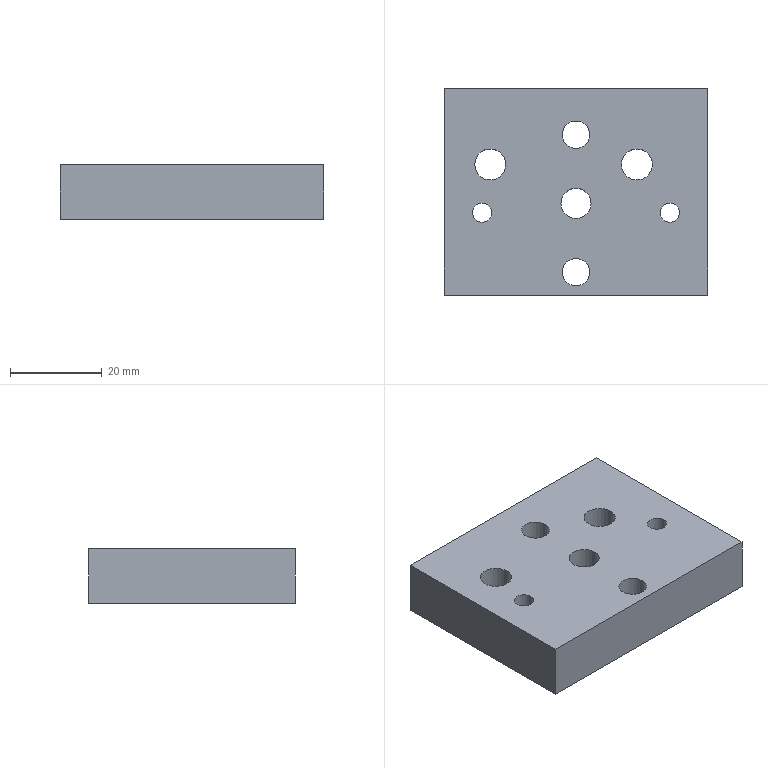Part | NX | features BREP 1 | 1 solid | 15 faces | box 57.5 x 45 x 12 mm | volume 28368 mm3 | cylinder 8 | plane 7 | commonest cylinder face diameters 4.2 x2 6 x2 6.8 x2 6.6 x1 11 x1
STEP:
#1=CARTESIAN_POINT('',(28.75,-22.5,0.));
#2=VERTEX_POINT('',#1);
#3=CARTESIAN_POINT('',(28.75,22.5,0.));
#4=VERTEX_POINT('',#3);
#5=CARTESIAN_POINT('',(28.75,22.5,0.));
#6=DIRECTION('',(0.,1.,0.));
#7=VECTOR('',#6,1000.);
#8=LINE('',#5,#7);
#9=EDGE_CURVE('',#2,#4,#8,.T.);
#10=ORIENTED_EDGE('',*,*,#9,.T.);
#11=CARTESIAN_POINT('',(28.75,22.5,12.));
#12=VERTEX_POINT('',#11);
#13=CARTESIAN_POINT('',(28.75,22.5,12.));
#14=DIRECTION('',(0.,0.,-1.));
#15=VECTOR('',#14,1000.);
#16=LINE('',#13,#15);
#17=EDGE_CURVE('',#12,#4,#16,.T.);
#18=ORIENTED_EDGE('',*,*,#17,.F.);
#19=CARTESIAN_POINT('',(28.75,-22.5,12.));
#20=VERTEX_POINT('',#19);
#21=CARTESIAN_POINT('',(28.75,22.5,12.));
#22=DIRECTION('',(0.,1.,0.));
#23=VECTOR('',#22,1000.);
#24=LINE('',#21,#23);
#25=EDGE_CURVE('',#20,#12,#24,.T.);
#26=ORIENTED_EDGE('',*,*,#25,.F.);
#27=CARTESIAN_POINT('',(28.75,-22.5,12.));
#28=DIRECTION('',(0.,0.,-1.));
#29=VECTOR('',#28,1000.);
#30=LINE('',#27,#29);
#31=EDGE_CURVE('',#20,#2,#30,.T.);
#32=ORIENTED_EDGE('',*,*,#31,.T.);
#33=EDGE_LOOP('',(#10,#18,#26,#32));
#34=FACE_BOUND('',#33,.T.);
#35=CARTESIAN_POINT('',(28.75,22.5,12.));
#36=DIRECTION('',(-1.,0.,0.));
#37=DIRECTION('',(0.,1.,0.));
#38=AXIS2_PLACEMENT_3D('',#35,#36,#37);
#39=PLANE('',#38);
#40=ADVANCED_FACE('',(#34),#39,.F.);
#41=CARTESIAN_POINT('',(-28.75,22.5,0.));
#42=VERTEX_POINT('',#41);
#43=CARTESIAN_POINT('',(-28.75,22.5,0.));
#44=DIRECTION('',(-1.,0.,0.));
#45=VECTOR('',#44,1000.);
#46=LINE('',#43,#45);
#47=EDGE_CURVE('',#4,#42,#46,.T.);
#48=ORIENTED_EDGE('',*,*,#47,.T.);
#49=CARTESIAN_POINT('',(-28.75,22.5,12.));
#50=VERTEX_POINT('',#49);
#51=CARTESIAN_POINT('',(-28.75,22.5,12.));
#52=DIRECTION('',(0.,0.,-1.));
#53=VECTOR('',#52,1000.);
#54=LINE('',#51,#53);
#55=EDGE_CURVE('',#50,#42,#54,.T.);
#56=ORIENTED_EDGE('',*,*,#55,.F.);
#57=CARTESIAN_POINT('',(-28.75,22.5,12.));
#58=DIRECTION('',(-1.,0.,0.));
#59=VECTOR('',#58,1000.);
#60=LINE('',#57,#59);
#61=EDGE_CURVE('',#12,#50,#60,.T.);
#62=ORIENTED_EDGE('',*,*,#61,.F.);
#63=ORIENTED_EDGE('',*,*,#17,.T.);
#64=EDGE_LOOP('',(#48,#56,#62,#63));
#65=FACE_BOUND('',#64,.T.);
#66=CARTESIAN_POINT('',(-28.75,22.5,12.));
#67=DIRECTION('',(0.,-1.,0.));
#68=DIRECTION('',(0.,0.,1.));
#69=AXIS2_PLACEMENT_3D('',#66,#67,#68);
#70=PLANE('',#69);
#71=ADVANCED_FACE('',(#65),#70,.F.);
#72=CARTESIAN_POINT('',(-28.75,-22.5,0.));
#73=VERTEX_POINT('',#72);
#74=CARTESIAN_POINT('',(-28.75,22.5,0.));
#75=DIRECTION('',(0.,-1.,0.));
#76=VECTOR('',#75,1000.);
#77=LINE('',#74,#76);
#78=EDGE_CURVE('',#42,#73,#77,.T.);
#79=ORIENTED_EDGE('',*,*,#78,.T.);
#80=CARTESIAN_POINT('',(-28.75,-22.5,12.));
#81=VERTEX_POINT('',#80);
#82=CARTESIAN_POINT('',(-28.75,-22.5,12.));
#83=DIRECTION('',(0.,0.,-1.));
#84=VECTOR('',#83,1000.);
#85=LINE('',#82,#84);
#86=EDGE_CURVE('',#81,#73,#85,.T.);
#87=ORIENTED_EDGE('',*,*,#86,.F.);
#88=CARTESIAN_POINT('',(-28.75,22.5,12.));
#89=DIRECTION('',(0.,-1.,0.));
#90=VECTOR('',#89,1000.);
#91=LINE('',#88,#90);
#92=EDGE_CURVE('',#50,#81,#91,.T.);
#93=ORIENTED_EDGE('',*,*,#92,.F.);
#94=ORIENTED_EDGE('',*,*,#55,.T.);
#95=EDGE_LOOP('',(#79,#87,#93,#94));
#96=FACE_BOUND('',#95,.T.);
#97=CARTESIAN_POINT('',(-28.75,22.5,12.));
#98=DIRECTION('',(1.,0.,0.));
#99=DIRECTION('',(0.,-1.,0.));
#100=AXIS2_PLACEMENT_3D('',#97,#98,#99);
#101=PLANE('',#100);
#102=ADVANCED_FACE('',(#96),#101,.F.);
#103=CARTESIAN_POINT('',(-28.75,-22.5,0.));
#104=DIRECTION('',(1.,0.,0.));
#105=VECTOR('',#104,1000.);
#106=LINE('',#103,#105);
#107=EDGE_CURVE('',#73,#2,#106,.T.);
#108=ORIENTED_EDGE('',*,*,#107,.T.);
#109=ORIENTED_EDGE('',*,*,#31,.F.);
#110=CARTESIAN_POINT('',(-28.75,-22.5,12.));
#111=DIRECTION('',(1.,0.,0.));
#112=VECTOR('',#111,1000.);
#113=LINE('',#110,#112);
#114=EDGE_CURVE('',#81,#20,#113,.T.);
#115=ORIENTED_EDGE('',*,*,#114,.F.);
#116=ORIENTED_EDGE('',*,*,#86,.T.);
#117=EDGE_LOOP('',(#108,#109,#115,#116));
#118=FACE_BOUND('',#117,.T.);
#119=CARTESIAN_POINT('',(-28.75,-22.5,12.));
#120=DIRECTION('',(0.,1.,0.));
#121=DIRECTION('',(0.,0.,-1.));
#122=AXIS2_PLACEMENT_3D('',#119,#120,#121);
#123=PLANE('',#122);
#124=ADVANCED_FACE('',(#118),#123,.F.);
#125=CARTESIAN_POINT('',(-3.3,-2.5,12.));
#126=VERTEX_POINT('',#125);
#127=CARTESIAN_POINT('',(0.,-2.5,12.));
#128=DIRECTION('',(0.,0.,-1.));
#129=DIRECTION('',(-1.,0.,0.));
#130=AXIS2_PLACEMENT_3D('',#127,#128,#129);
#131=CIRCLE('',#130,3.3);
#132=EDGE_CURVE('',#126,#126,#131,.T.);
#133=ORIENTED_EDGE('',*,*,#132,.T.);
#134=EDGE_LOOP('',(#133));
#135=FACE_BOUND('',#134,.T.);
#136=CARTESIAN_POINT('',(-3.,-17.5,12.));
#137=VERTEX_POINT('',#136);
#138=CARTESIAN_POINT('',(0.,-17.5,12.));
#139=DIRECTION('',(0.,0.,-1.));
#140=DIRECTION('',(-1.,0.,0.));
#141=AXIS2_PLACEMENT_3D('',#138,#139,#140);
#142=CIRCLE('',#141,3.);
#143=EDGE_CURVE('',#137,#137,#142,.T.);
#144=ORIENTED_EDGE('',*,*,#143,.T.);
#145=EDGE_LOOP('',(#144));
#146=FACE_BOUND('',#145,.T.);
#147=CARTESIAN_POINT('',(-3.,12.5,12.));
#148=VERTEX_POINT('',#147);
#149=CARTESIAN_POINT('',(0.,12.5,12.));
#150=DIRECTION('',(0.,0.,-1.));
#151=DIRECTION('',(-1.,0.,0.));
#152=AXIS2_PLACEMENT_3D('',#149,#150,#151);
#153=CIRCLE('',#152,3.);
#154=EDGE_CURVE('',#148,#148,#153,.T.);
#155=ORIENTED_EDGE('',*,*,#154,.T.);
#156=EDGE_LOOP('',(#155));
#157=FACE_BOUND('',#156,.T.);
#158=CARTESIAN_POINT('',(-18.4,-4.5,12.));
#159=VERTEX_POINT('',#158);
#160=CARTESIAN_POINT('',(-20.5,-4.5,12.));
#161=DIRECTION('',(0.,0.,1.));
#162=DIRECTION('',(1.,0.,0.));
#163=AXIS2_PLACEMENT_3D('',#160,#161,#162);
#164=CIRCLE('',#163,2.1);
#165=EDGE_CURVE('',#159,#159,#164,.T.);
#166=ORIENTED_EDGE('',*,*,#165,.F.);
#167=EDGE_LOOP('',(#166));
#168=FACE_BOUND('',#167,.T.);
#169=CARTESIAN_POINT('',(22.6,-4.5,12.));
#170=VERTEX_POINT('',#169);
#171=CARTESIAN_POINT('',(20.5,-4.5,12.));
#172=DIRECTION('',(0.,0.,1.));
#173=DIRECTION('',(1.,0.,0.));
#174=AXIS2_PLACEMENT_3D('',#171,#172,#173);
#175=CIRCLE('',#174,2.1);
#176=EDGE_CURVE('',#170,#170,#175,.T.);
#177=ORIENTED_EDGE('',*,*,#176,.F.);
#178=EDGE_LOOP('',(#177));
#179=FACE_BOUND('',#178,.T.);
#180=CARTESIAN_POINT('',(9.886,6.,12.));
#181=VERTEX_POINT('',#180);
#182=CARTESIAN_POINT('',(13.286,6.,12.));
#183=DIRECTION('',(0.,0.,-1.));
#184=DIRECTION('',(-1.,0.,0.));
#185=AXIS2_PLACEMENT_3D('',#182,#183,#184);
#186=CIRCLE('',#185,3.4);
#187=EDGE_CURVE('',#181,#181,#186,.T.);
#188=ORIENTED_EDGE('',*,*,#187,.T.);
#189=EDGE_LOOP('',(#188));
#190=FACE_BOUND('',#189,.T.);
#191=CARTESIAN_POINT('',(-22.114,6.,12.));
#192=VERTEX_POINT('',#191);
#193=CARTESIAN_POINT('',(-18.714,6.,12.));
#194=DIRECTION('',(0.,0.,-1.));
#195=DIRECTION('',(-1.,0.,0.));
#196=AXIS2_PLACEMENT_3D('',#193,#194,#195);
#197=CIRCLE('',#196,3.4);
#198=EDGE_CURVE('',#192,#192,#197,.T.);
#199=ORIENTED_EDGE('',*,*,#198,.T.);
#200=EDGE_LOOP('',(#199));
#201=FACE_BOUND('',#200,.T.);
#202=ORIENTED_EDGE('',*,*,#25,.T.);
#203=ORIENTED_EDGE('',*,*,#61,.T.);
#204=ORIENTED_EDGE('',*,*,#92,.T.);
#205=ORIENTED_EDGE('',*,*,#114,.T.);
#206=EDGE_LOOP('',(#202,#203,#204,#205));
#207=FACE_BOUND('',#206,.T.);
#208=CARTESIAN_POINT('',(0.,0.,12.));
#209=DIRECTION('',(0.,0.,1.));
#210=DIRECTION('',(-1.,0.,0.));
#211=AXIS2_PLACEMENT_3D('',#208,#209,#210);
#212=PLANE('',#211);
#213=ADVANCED_FACE('',(#135,#146,#157,#168,#179,#190,#201,#207),#212,.T.);
#214=CARTESIAN_POINT('',(-5.5,-2.5,0.));
#215=VERTEX_POINT('',#214);
#216=CARTESIAN_POINT('',(0.,-2.5,0.));
#217=DIRECTION('',(0.,0.,-1.));
#218=DIRECTION('',(-1.,0.,0.));
#219=AXIS2_PLACEMENT_3D('',#216,#217,#218);
#220=CIRCLE('',#219,5.5);
#221=EDGE_CURVE('',#215,#215,#220,.T.);
#222=ORIENTED_EDGE('',*,*,#221,.F.);
#223=EDGE_LOOP('',(#222));
#224=FACE_BOUND('',#223,.T.);
#225=CARTESIAN_POINT('',(-3.,-17.5,0.));
#226=VERTEX_POINT('',#225);
#227=CARTESIAN_POINT('',(0.,-17.5,0.));
#228=DIRECTION('',(0.,0.,-1.));
#229=DIRECTION('',(-1.,0.,0.));
#230=AXIS2_PLACEMENT_3D('',#227,#228,#229);
#231=CIRCLE('',#230,3.);
#232=EDGE_CURVE('',#226,#226,#231,.T.);
#233=ORIENTED_EDGE('',*,*,#232,.F.);
#234=EDGE_LOOP('',(#233));
#235=FACE_BOUND('',#234,.T.);
#236=CARTESIAN_POINT('',(-3.,12.5,0.));
#237=VERTEX_POINT('',#236);
#238=CARTESIAN_POINT('',(0.,12.5,0.));
#239=DIRECTION('',(0.,0.,-1.));
#240=DIRECTION('',(-1.,0.,0.));
#241=AXIS2_PLACEMENT_3D('',#238,#239,#240);
#242=CIRCLE('',#241,3.);
#243=EDGE_CURVE('',#237,#237,#242,.T.);
#244=ORIENTED_EDGE('',*,*,#243,.F.);
#245=EDGE_LOOP('',(#244));
#246=FACE_BOUND('',#245,.T.);
#247=CARTESIAN_POINT('',(-18.4,-4.5,0.));
#248=VERTEX_POINT('',#247);
#249=CARTESIAN_POINT('',(-20.5,-4.5,0.));
#250=DIRECTION('',(0.,0.,1.));
#251=DIRECTION('',(1.,0.,0.));
#252=AXIS2_PLACEMENT_3D('',#249,#250,#251);
#253=CIRCLE('',#252,2.1);
#254=EDGE_CURVE('',#248,#248,#253,.T.);
#255=ORIENTED_EDGE('',*,*,#254,.T.);
#256=EDGE_LOOP('',(#255));
#257=FACE_BOUND('',#256,.T.);
#258=CARTESIAN_POINT('',(22.6,-4.5,0.));
#259=VERTEX_POINT('',#258);
#260=CARTESIAN_POINT('',(20.5,-4.5,0.));
#261=DIRECTION('',(0.,0.,1.));
#262=DIRECTION('',(1.,0.,0.));
#263=AXIS2_PLACEMENT_3D('',#260,#261,#262);
#264=CIRCLE('',#263,2.1);
#265=EDGE_CURVE('',#259,#259,#264,.T.);
#266=ORIENTED_EDGE('',*,*,#265,.T.);
#267=EDGE_LOOP('',(#266));
#268=FACE_BOUND('',#267,.T.);
#269=CARTESIAN_POINT('',(9.886,6.,0.));
#270=VERTEX_POINT('',#269);
#271=CARTESIAN_POINT('',(13.286,6.,0.));
#272=DIRECTION('',(0.,0.,-1.));
#273=DIRECTION('',(-1.,0.,0.));
#274=AXIS2_PLACEMENT_3D('',#271,#272,#273);
#275=CIRCLE('',#274,3.4);
#276=EDGE_CURVE('',#270,#270,#275,.T.);
#277=ORIENTED_EDGE('',*,*,#276,.F.);
#278=EDGE_LOOP('',(#277));
#279=FACE_BOUND('',#278,.T.);
#280=CARTESIAN_POINT('',(-22.114,6.,0.));
#281=VERTEX_POINT('',#280);
#282=CARTESIAN_POINT('',(-18.714,6.,0.));
#283=DIRECTION('',(0.,0.,-1.));
#284=DIRECTION('',(-1.,0.,0.));
#285=AXIS2_PLACEMENT_3D('',#282,#283,#284);
#286=CIRCLE('',#285,3.4);
#287=EDGE_CURVE('',#281,#281,#286,.T.);
#288=ORIENTED_EDGE('',*,*,#287,.F.);
#289=EDGE_LOOP('',(#288));
#290=FACE_BOUND('',#289,.T.);
#291=ORIENTED_EDGE('',*,*,#9,.F.);
#292=ORIENTED_EDGE('',*,*,#107,.F.);
#293=ORIENTED_EDGE('',*,*,#78,.F.);
#294=ORIENTED_EDGE('',*,*,#47,.F.);
#295=EDGE_LOOP('',(#291,#292,#293,#294));
#296=FACE_BOUND('',#295,.T.);
#297=CARTESIAN_POINT('',(0.,0.,0.));
#298=DIRECTION('',(0.,0.,1.));
#299=DIRECTION('',(-1.,0.,0.));
#300=AXIS2_PLACEMENT_3D('',#297,#298,#299);
#301=PLANE('',#300);
#302=ADVANCED_FACE('',(#224,#235,#246,#257,#268,#279,#290,#296),#301,.F.);
#303=ORIENTED_EDGE('',*,*,#198,.F.);
#304=EDGE_LOOP('',(#303));
#305=FACE_BOUND('',#304,.T.);
#306=ORIENTED_EDGE('',*,*,#287,.T.);
#307=EDGE_LOOP('',(#306));
#308=FACE_BOUND('',#307,.T.);
#309=CARTESIAN_POINT('',(-18.714,6.,0.));
#310=DIRECTION('',(0.,0.,-1.));
#311=DIRECTION('',(1.,0.,0.));
#312=AXIS2_PLACEMENT_3D('',#309,#310,#311);
#313=CYLINDRICAL_SURFACE('',#312,3.4);
#314=ADVANCED_FACE('',(#305,#308),#313,.F.);
#315=ORIENTED_EDGE('',*,*,#187,.F.);
#316=EDGE_LOOP('',(#315));
#317=FACE_BOUND('',#316,.T.);
#318=ORIENTED_EDGE('',*,*,#276,.T.);
#319=EDGE_LOOP('',(#318));
#320=FACE_BOUND('',#319,.T.);
#321=CARTESIAN_POINT('',(13.286,6.,0.));
#322=DIRECTION('',(0.,0.,-1.));
#323=DIRECTION('',(1.,0.,0.));
#324=AXIS2_PLACEMENT_3D('',#321,#322,#323);
#325=CYLINDRICAL_SURFACE('',#324,3.4);
#326=ADVANCED_FACE('',(#317,#320),#325,.F.);
#327=ORIENTED_EDGE('',*,*,#265,.F.);
#328=EDGE_LOOP('',(#327));
#329=FACE_BOUND('',#328,.T.);
#330=ORIENTED_EDGE('',*,*,#176,.T.);
#331=EDGE_LOOP('',(#330));
#332=FACE_BOUND('',#331,.T.);
#333=CARTESIAN_POINT('',(20.5,-4.5,12.));
#334=DIRECTION('',(0.,0.,1.));
#335=DIRECTION('',(-1.,0.,0.));
#336=AXIS2_PLACEMENT_3D('',#333,#334,#335);
#337=CYLINDRICAL_SURFACE('',#336,2.1);
#338=ADVANCED_FACE('',(#329,#332),#337,.F.);
#339=ORIENTED_EDGE('',*,*,#254,.F.);
#340=EDGE_LOOP('',(#339));
#341=FACE_BOUND('',#340,.T.);
#342=ORIENTED_EDGE('',*,*,#165,.T.);
#343=EDGE_LOOP('',(#342));
#344=FACE_BOUND('',#343,.T.);
#345=CARTESIAN_POINT('',(-20.5,-4.5,12.));
#346=DIRECTION('',(0.,0.,1.));
#347=DIRECTION('',(-1.,0.,0.));
#348=AXIS2_PLACEMENT_3D('',#345,#346,#347);
#349=CYLINDRICAL_SURFACE('',#348,2.1);
#350=ADVANCED_FACE('',(#341,#344),#349,.F.);
#351=ORIENTED_EDGE('',*,*,#154,.F.);
#352=EDGE_LOOP('',(#351));
#353=FACE_BOUND('',#352,.T.);
#354=ORIENTED_EDGE('',*,*,#243,.T.);
#355=EDGE_LOOP('',(#354));
#356=FACE_BOUND('',#355,.T.);
#357=CARTESIAN_POINT('',(0.,12.5,0.));
#358=DIRECTION('',(0.,0.,-1.));
#359=DIRECTION('',(1.,0.,0.));
#360=AXIS2_PLACEMENT_3D('',#357,#358,#359);
#361=CYLINDRICAL_SURFACE('',#360,3.);
#362=ADVANCED_FACE('',(#353,#356),#361,.F.);
#363=ORIENTED_EDGE('',*,*,#143,.F.);
#364=EDGE_LOOP('',(#363));
#365=FACE_BOUND('',#364,.T.);
#366=ORIENTED_EDGE('',*,*,#232,.T.);
#367=EDGE_LOOP('',(#366));
#368=FACE_BOUND('',#367,.T.);
#369=CARTESIAN_POINT('',(0.,-17.5,0.));
#370=DIRECTION('',(0.,0.,-1.));
#371=DIRECTION('',(1.,0.,0.));
#372=AXIS2_PLACEMENT_3D('',#369,#370,#371);
#373=CYLINDRICAL_SURFACE('',#372,3.);
#374=ADVANCED_FACE('',(#365,#368),#373,.F.);
#375=ORIENTED_EDGE('',*,*,#132,.F.);
#376=EDGE_LOOP('',(#375));
#377=FACE_BOUND('',#376,.T.);
#378=CARTESIAN_POINT('',(-3.3,-2.5,6.4));
#379=VERTEX_POINT('',#378);
#380=CARTESIAN_POINT('',(0.,-2.5,6.4));
#381=DIRECTION('',(0.,0.,-1.));
#382=DIRECTION('',(-1.,0.,0.));
#383=AXIS2_PLACEMENT_3D('',#380,#381,#382);
#384=CIRCLE('',#383,3.3);
#385=EDGE_CURVE('',#379,#379,#384,.T.);
#386=ORIENTED_EDGE('',*,*,#385,.T.);
#387=EDGE_LOOP('',(#386));
#388=FACE_BOUND('',#387,.T.);
#389=CARTESIAN_POINT('',(0.,-2.5,0.));
#390=DIRECTION('',(0.,0.,-1.));
#391=DIRECTION('',(1.,0.,0.));
#392=AXIS2_PLACEMENT_3D('',#389,#390,#391);
#393=CYLINDRICAL_SURFACE('',#392,3.3);
#394=ADVANCED_FACE('',(#377,#388),#393,.F.);
#395=ORIENTED_EDGE('',*,*,#385,.F.);
#396=EDGE_LOOP('',(#395));
#397=FACE_BOUND('',#396,.T.);
#398=CARTESIAN_POINT('',(-5.5,-2.5,6.4));
#399=VERTEX_POINT('',#398);
#400=CARTESIAN_POINT('',(0.,-2.5,6.4));
#401=DIRECTION('',(0.,0.,-1.));
#402=DIRECTION('',(-1.,0.,0.));
#403=AXIS2_PLACEMENT_3D('',#400,#401,#402);
#404=CIRCLE('',#403,5.5);
#405=EDGE_CURVE('',#399,#399,#404,.T.);
#406=ORIENTED_EDGE('',*,*,#405,.T.);
#407=EDGE_LOOP('',(#406));
#408=FACE_BOUND('',#407,.T.);
#409=CARTESIAN_POINT('',(3.3,-2.5,6.4));
#410=DIRECTION('',(0.,0.,1.));
#411=DIRECTION('',(-1.,0.,0.));
#412=AXIS2_PLACEMENT_3D('',#409,#410,#411);
#413=PLANE('',#412);
#414=ADVANCED_FACE('',(#397,#408),#413,.F.);
#415=ORIENTED_EDGE('',*,*,#405,.F.);
#416=EDGE_LOOP('',(#415));
#417=FACE_BOUND('',#416,.T.);
#418=ORIENTED_EDGE('',*,*,#221,.T.);
#419=EDGE_LOOP('',(#418));
#420=FACE_BOUND('',#419,.T.);
#421=CARTESIAN_POINT('',(0.,-2.5,0.));
#422=DIRECTION('',(0.,0.,-1.));
#423=DIRECTION('',(1.,0.,0.));
#424=AXIS2_PLACEMENT_3D('',#421,#422,#423);
#425=CYLINDRICAL_SURFACE('',#424,5.5);
#426=ADVANCED_FACE('',(#417,#420),#425,.F.);
#427=CLOSED_SHELL('',(#40,#71,#102,#124,#213,#302,#314,#326,#338,#350,#362,#374,#394,#414,#426));
#428=MANIFOLD_SOLID_BREP('',#427);
#429=(LENGTH_UNIT()NAMED_UNIT(*)SI_UNIT(.MILLI.,.METRE.));
#430=UNCERTAINTY_MEASURE_WITH_UNIT(LENGTH_MEASURE(0.00001),#429,'','');
#431=(NAMED_UNIT(*)PLANE_ANGLE_UNIT()SI_UNIT($,.RADIAN.));
#432=(NAMED_UNIT(*)SI_UNIT($,.STERADIAN.)SOLID_ANGLE_UNIT());
#433=(GEOMETRIC_REPRESENTATION_CONTEXT(3)GLOBAL_UNCERTAINTY_ASSIGNED_CONTEXT((#430))GLOBAL_UNIT_ASSIGNED_CONTEXT((#429,#431,#432))REPRESENTATION_CONTEXT('',''));
#434=ADVANCED_BREP_SHAPE_REPRESENTATION('',(#428),#433);